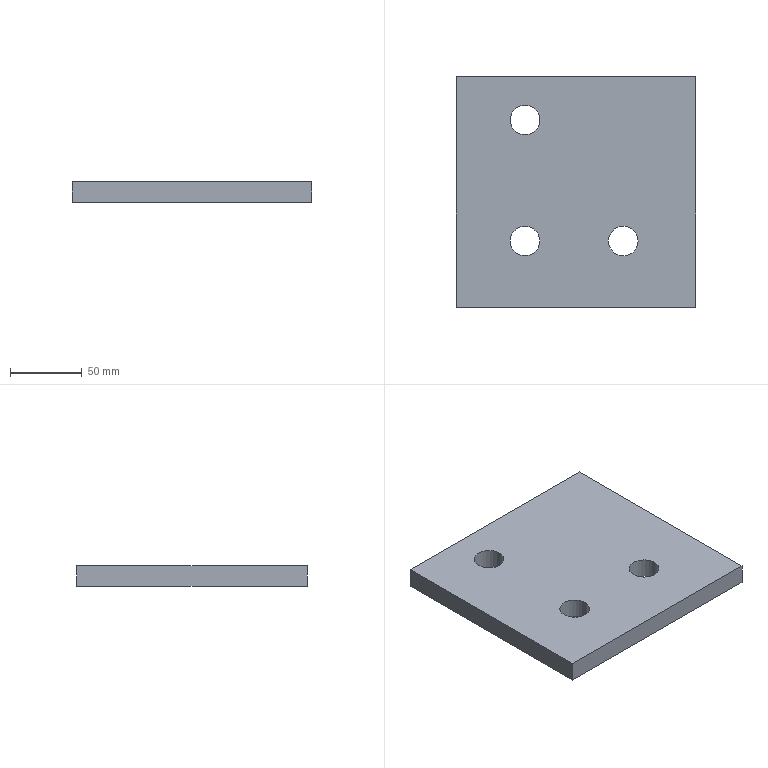Part | SolidWorks | features Extrusion 1 | 1 solid | 12 faces | box 166.35 x 160 x 14 mm | volume 358558 mm3 | cylinder 6 | plane 6 | commonest cylinder face diameters 20.65 x6
STEP:
#1=CARTESIAN_POINT('',(22.527,-34.102,14.));
#2=VERTEX_POINT('',#1);
#3=CARTESIAN_POINT('',(43.177,-34.102,14.));
#4=VERTEX_POINT('',#3);
#5=CARTESIAN_POINT('',(32.852,-34.102,14.));
#6=DIRECTION('',(0.,0.,1.));
#7=DIRECTION('',(1.,0.,0.));
#8=AXIS2_PLACEMENT_3D('',#5,#6,#7);
#9=CIRCLE('',#8,10.325);
#10=EDGE_CURVE('',#2,#4,#9,.T.);
#11=ORIENTED_EDGE('',*,*,#10,.T.);
#12=CARTESIAN_POINT('',(43.177,-34.102,0.));
#13=VERTEX_POINT('',#12);
#14=CARTESIAN_POINT('',(43.177,-34.102,14.));
#15=DIRECTION('',(0.,0.,-1.));
#16=VECTOR('',#15,1000.);
#17=LINE('',#14,#16);
#18=EDGE_CURVE('',#4,#13,#17,.T.);
#19=ORIENTED_EDGE('',*,*,#18,.T.);
#20=CARTESIAN_POINT('',(22.527,-34.102,0.));
#21=VERTEX_POINT('',#20);
#22=CARTESIAN_POINT('',(32.852,-34.102,0.));
#23=DIRECTION('',(0.,0.,1.));
#24=DIRECTION('',(1.,0.,0.));
#25=AXIS2_PLACEMENT_3D('',#22,#23,#24);
#26=CIRCLE('',#25,10.325);
#27=EDGE_CURVE('',#21,#13,#26,.T.);
#28=ORIENTED_EDGE('',*,*,#27,.F.);
#29=CARTESIAN_POINT('',(22.527,-34.102,14.));
#30=DIRECTION('',(0.,0.,-1.));
#31=VECTOR('',#30,1000.);
#32=LINE('',#29,#31);
#33=EDGE_CURVE('',#2,#21,#32,.T.);
#34=ORIENTED_EDGE('',*,*,#33,.F.);
#35=EDGE_LOOP('',(#11,#19,#28,#34));
#36=FACE_OUTER_BOUND('',#35,.T.);
#37=CARTESIAN_POINT('',(32.852,-34.102,14.));
#38=DIRECTION('',(0.,0.,-1.));
#39=DIRECTION('',(-1.,0.,0.));
#40=AXIS2_PLACEMENT_3D('',#37,#38,#39);
#41=CYLINDRICAL_SURFACE('',#40,10.325);
#42=ADVANCED_FACE('',(#36),#41,.F.);
#43=CARTESIAN_POINT('',(-45.78,-34.102,14.));
#44=VERTEX_POINT('',#43);
#45=CARTESIAN_POINT('',(-25.13,-34.102,14.));
#46=VERTEX_POINT('',#45);
#47=CARTESIAN_POINT('',(-35.455,-34.102,14.));
#48=DIRECTION('',(0.,0.,1.));
#49=DIRECTION('',(1.,0.,0.));
#50=AXIS2_PLACEMENT_3D('',#47,#48,#49);
#51=CIRCLE('',#50,10.325);
#52=EDGE_CURVE('',#44,#46,#51,.T.);
#53=ORIENTED_EDGE('',*,*,#52,.T.);
#54=CARTESIAN_POINT('',(-25.13,-34.102,0.));
#55=VERTEX_POINT('',#54);
#56=CARTESIAN_POINT('',(-25.13,-34.102,14.));
#57=DIRECTION('',(0.,0.,-1.));
#58=VECTOR('',#57,1000.);
#59=LINE('',#56,#58);
#60=EDGE_CURVE('',#46,#55,#59,.T.);
#61=ORIENTED_EDGE('',*,*,#60,.T.);
#62=CARTESIAN_POINT('',(-45.78,-34.102,0.));
#63=VERTEX_POINT('',#62);
#64=CARTESIAN_POINT('',(-35.455,-34.102,0.));
#65=DIRECTION('',(0.,0.,1.));
#66=DIRECTION('',(1.,0.,0.));
#67=AXIS2_PLACEMENT_3D('',#64,#65,#66);
#68=CIRCLE('',#67,10.325);
#69=EDGE_CURVE('',#63,#55,#68,.T.);
#70=ORIENTED_EDGE('',*,*,#69,.F.);
#71=CARTESIAN_POINT('',(-45.78,-34.102,14.));
#72=DIRECTION('',(0.,0.,-1.));
#73=VECTOR('',#72,1000.);
#74=LINE('',#71,#73);
#75=EDGE_CURVE('',#44,#63,#74,.T.);
#76=ORIENTED_EDGE('',*,*,#75,.F.);
#77=EDGE_LOOP('',(#53,#61,#70,#76));
#78=FACE_OUTER_BOUND('',#77,.T.);
#79=CARTESIAN_POINT('',(-35.455,-34.102,14.));
#80=DIRECTION('',(0.,0.,-1.));
#81=DIRECTION('',(-1.,0.,0.));
#82=AXIS2_PLACEMENT_3D('',#79,#80,#81);
#83=CYLINDRICAL_SURFACE('',#82,10.325);
#84=ADVANCED_FACE('',(#78),#83,.F.);
#85=CARTESIAN_POINT('',(-45.748,50.048,14.));
#86=VERTEX_POINT('',#85);
#87=CARTESIAN_POINT('',(-25.098,50.048,14.));
#88=VERTEX_POINT('',#87);
#89=CARTESIAN_POINT('',(-35.423,50.048,14.));
#90=DIRECTION('',(0.,0.,1.));
#91=DIRECTION('',(1.,0.,0.));
#92=AXIS2_PLACEMENT_3D('',#89,#90,#91);
#93=CIRCLE('',#92,10.325);
#94=EDGE_CURVE('',#86,#88,#93,.T.);
#95=ORIENTED_EDGE('',*,*,#94,.T.);
#96=CARTESIAN_POINT('',(-25.098,50.048,0.));
#97=VERTEX_POINT('',#96);
#98=CARTESIAN_POINT('',(-25.098,50.048,14.));
#99=DIRECTION('',(0.,0.,-1.));
#100=VECTOR('',#99,1000.);
#101=LINE('',#98,#100);
#102=EDGE_CURVE('',#88,#97,#101,.T.);
#103=ORIENTED_EDGE('',*,*,#102,.T.);
#104=CARTESIAN_POINT('',(-45.748,50.048,0.));
#105=VERTEX_POINT('',#104);
#106=CARTESIAN_POINT('',(-35.423,50.048,0.));
#107=DIRECTION('',(0.,0.,1.));
#108=DIRECTION('',(1.,0.,0.));
#109=AXIS2_PLACEMENT_3D('',#106,#107,#108);
#110=CIRCLE('',#109,10.325);
#111=EDGE_CURVE('',#105,#97,#110,.T.);
#112=ORIENTED_EDGE('',*,*,#111,.F.);
#113=CARTESIAN_POINT('',(-45.748,50.048,14.));
#114=DIRECTION('',(0.,0.,-1.));
#115=VECTOR('',#114,1000.);
#116=LINE('',#113,#115);
#117=EDGE_CURVE('',#86,#105,#116,.T.);
#118=ORIENTED_EDGE('',*,*,#117,.F.);
#119=EDGE_LOOP('',(#95,#103,#112,#118));
#120=FACE_OUTER_BOUND('',#119,.T.);
#121=CARTESIAN_POINT('',(-35.423,50.048,14.));
#122=DIRECTION('',(0.,0.,-1.));
#123=DIRECTION('',(-1.,0.,0.));
#124=AXIS2_PLACEMENT_3D('',#121,#122,#123);
#125=CYLINDRICAL_SURFACE('',#124,10.325);
#126=ADVANCED_FACE('',(#120),#125,.F.);
#127=ORIENTED_EDGE('',*,*,#52,.F.);
#128=CARTESIAN_POINT('',(-35.455,-34.102,14.));
#129=DIRECTION('',(0.,0.,1.));
#130=DIRECTION('',(1.,0.,0.));
#131=AXIS2_PLACEMENT_3D('',#128,#129,#130);
#132=CIRCLE('',#131,10.325);
#133=EDGE_CURVE('',#46,#44,#132,.T.);
#134=ORIENTED_EDGE('',*,*,#133,.F.);
#135=EDGE_LOOP('',(#127,#134));
#136=FACE_BOUND('',#135,.T.);
#137=CARTESIAN_POINT('',(83.175,-80.,14.));
#138=VERTEX_POINT('',#137);
#139=CARTESIAN_POINT('',(83.175,80.,14.));
#140=VERTEX_POINT('',#139);
#141=CARTESIAN_POINT('',(83.175,80.,14.));
#142=DIRECTION('',(0.,1.,0.));
#143=VECTOR('',#142,1000.);
#144=LINE('',#141,#143);
#145=EDGE_CURVE('',#138,#140,#144,.T.);
#146=ORIENTED_EDGE('',*,*,#145,.T.);
#147=CARTESIAN_POINT('',(-83.175,80.,14.));
#148=VERTEX_POINT('',#147);
#149=CARTESIAN_POINT('',(-83.175,80.,14.));
#150=DIRECTION('',(-1.,0.,0.));
#151=VECTOR('',#150,1000.);
#152=LINE('',#149,#151);
#153=EDGE_CURVE('',#140,#148,#152,.T.);
#154=ORIENTED_EDGE('',*,*,#153,.T.);
#155=CARTESIAN_POINT('',(-83.175,-80.,14.));
#156=VERTEX_POINT('',#155);
#157=CARTESIAN_POINT('',(-83.175,80.,14.));
#158=DIRECTION('',(0.,-1.,0.));
#159=VECTOR('',#158,1000.);
#160=LINE('',#157,#159);
#161=EDGE_CURVE('',#148,#156,#160,.T.);
#162=ORIENTED_EDGE('',*,*,#161,.T.);
#163=CARTESIAN_POINT('',(-83.175,-80.,14.));
#164=DIRECTION('',(1.,0.,0.));
#165=VECTOR('',#164,1000.);
#166=LINE('',#163,#165);
#167=EDGE_CURVE('',#156,#138,#166,.T.);
#168=ORIENTED_EDGE('',*,*,#167,.T.);
#169=EDGE_LOOP('',(#146,#154,#162,#168));
#170=FACE_OUTER_BOUND('',#169,.T.);
#171=ORIENTED_EDGE('',*,*,#94,.F.);
#172=CARTESIAN_POINT('',(-35.423,50.048,14.));
#173=DIRECTION('',(0.,0.,1.));
#174=DIRECTION('',(1.,0.,0.));
#175=AXIS2_PLACEMENT_3D('',#172,#173,#174);
#176=CIRCLE('',#175,10.325);
#177=EDGE_CURVE('',#88,#86,#176,.T.);
#178=ORIENTED_EDGE('',*,*,#177,.F.);
#179=EDGE_LOOP('',(#171,#178));
#180=FACE_BOUND('',#179,.T.);
#181=ORIENTED_EDGE('',*,*,#10,.F.);
#182=CARTESIAN_POINT('',(32.852,-34.102,14.));
#183=DIRECTION('',(0.,0.,1.));
#184=DIRECTION('',(1.,0.,0.));
#185=AXIS2_PLACEMENT_3D('',#182,#183,#184);
#186=CIRCLE('',#185,10.325);
#187=EDGE_CURVE('',#4,#2,#186,.T.);
#188=ORIENTED_EDGE('',*,*,#187,.F.);
#189=EDGE_LOOP('',(#181,#188));
#190=FACE_BOUND('',#189,.T.);
#191=CARTESIAN_POINT('',(83.175,-80.,14.));
#192=DIRECTION('',(0.,0.,1.));
#193=DIRECTION('',(1.,0.,0.));
#194=AXIS2_PLACEMENT_3D('',#191,#192,#193);
#195=PLANE('',#194);
#196=ADVANCED_FACE('',(#136,#170,#180,#190),#195,.T.);
#197=ORIENTED_EDGE('',*,*,#69,.T.);
#198=CARTESIAN_POINT('',(-35.455,-34.102,0.));
#199=DIRECTION('',(0.,0.,1.));
#200=DIRECTION('',(1.,0.,0.));
#201=AXIS2_PLACEMENT_3D('',#198,#199,#200);
#202=CIRCLE('',#201,10.325);
#203=EDGE_CURVE('',#55,#63,#202,.T.);
#204=ORIENTED_EDGE('',*,*,#203,.T.);
#205=EDGE_LOOP('',(#197,#204));
#206=FACE_BOUND('',#205,.T.);
#207=CARTESIAN_POINT('',(83.175,-80.,0.));
#208=VERTEX_POINT('',#207);
#209=CARTESIAN_POINT('',(83.175,80.,0.));
#210=VERTEX_POINT('',#209);
#211=CARTESIAN_POINT('',(83.175,80.,0.));
#212=DIRECTION('',(0.,1.,0.));
#213=VECTOR('',#212,1000.);
#214=LINE('',#211,#213);
#215=EDGE_CURVE('',#208,#210,#214,.T.);
#216=ORIENTED_EDGE('',*,*,#215,.F.);
#217=CARTESIAN_POINT('',(-83.175,-80.,0.));
#218=VERTEX_POINT('',#217);
#219=CARTESIAN_POINT('',(-83.175,-80.,0.));
#220=DIRECTION('',(1.,0.,0.));
#221=VECTOR('',#220,1000.);
#222=LINE('',#219,#221);
#223=EDGE_CURVE('',#218,#208,#222,.T.);
#224=ORIENTED_EDGE('',*,*,#223,.F.);
#225=CARTESIAN_POINT('',(-83.175,80.,0.));
#226=VERTEX_POINT('',#225);
#227=CARTESIAN_POINT('',(-83.175,80.,0.));
#228=DIRECTION('',(0.,-1.,0.));
#229=VECTOR('',#228,1000.);
#230=LINE('',#227,#229);
#231=EDGE_CURVE('',#226,#218,#230,.T.);
#232=ORIENTED_EDGE('',*,*,#231,.F.);
#233=CARTESIAN_POINT('',(-83.175,80.,0.));
#234=DIRECTION('',(-1.,0.,0.));
#235=VECTOR('',#234,1000.);
#236=LINE('',#233,#235);
#237=EDGE_CURVE('',#210,#226,#236,.T.);
#238=ORIENTED_EDGE('',*,*,#237,.F.);
#239=EDGE_LOOP('',(#216,#224,#232,#238));
#240=FACE_OUTER_BOUND('',#239,.T.);
#241=ORIENTED_EDGE('',*,*,#111,.T.);
#242=CARTESIAN_POINT('',(-35.423,50.048,0.));
#243=DIRECTION('',(0.,0.,1.));
#244=DIRECTION('',(1.,0.,0.));
#245=AXIS2_PLACEMENT_3D('',#242,#243,#244);
#246=CIRCLE('',#245,10.325);
#247=EDGE_CURVE('',#97,#105,#246,.T.);
#248=ORIENTED_EDGE('',*,*,#247,.T.);
#249=EDGE_LOOP('',(#241,#248));
#250=FACE_BOUND('',#249,.T.);
#251=ORIENTED_EDGE('',*,*,#27,.T.);
#252=CARTESIAN_POINT('',(32.852,-34.102,0.));
#253=DIRECTION('',(0.,0.,1.));
#254=DIRECTION('',(1.,0.,0.));
#255=AXIS2_PLACEMENT_3D('',#252,#253,#254);
#256=CIRCLE('',#255,10.325);
#257=EDGE_CURVE('',#13,#21,#256,.T.);
#258=ORIENTED_EDGE('',*,*,#257,.T.);
#259=EDGE_LOOP('',(#251,#258));
#260=FACE_BOUND('',#259,.T.);
#261=CARTESIAN_POINT('',(83.175,-80.,0.));
#262=DIRECTION('',(0.,0.,1.));
#263=DIRECTION('',(1.,0.,0.));
#264=AXIS2_PLACEMENT_3D('',#261,#262,#263);
#265=PLANE('',#264);
#266=ADVANCED_FACE('',(#206,#240,#250,#260),#265,.F.);
#267=ORIENTED_EDGE('',*,*,#215,.T.);
#268=CARTESIAN_POINT('',(83.175,80.,14.));
#269=DIRECTION('',(0.,0.,-1.));
#270=VECTOR('',#269,1000.);
#271=LINE('',#268,#270);
#272=EDGE_CURVE('',#140,#210,#271,.T.);
#273=ORIENTED_EDGE('',*,*,#272,.F.);
#274=ORIENTED_EDGE('',*,*,#145,.F.);
#275=CARTESIAN_POINT('',(83.175,-80.,14.));
#276=DIRECTION('',(0.,0.,-1.));
#277=VECTOR('',#276,1000.);
#278=LINE('',#275,#277);
#279=EDGE_CURVE('',#138,#208,#278,.T.);
#280=ORIENTED_EDGE('',*,*,#279,.T.);
#281=EDGE_LOOP('',(#267,#273,#274,#280));
#282=FACE_OUTER_BOUND('',#281,.T.);
#283=CARTESIAN_POINT('',(83.175,80.,14.));
#284=DIRECTION('',(-1.,0.,0.));
#285=DIRECTION('',(0.,-1.,0.));
#286=AXIS2_PLACEMENT_3D('',#283,#284,#285);
#287=PLANE('',#286);
#288=ADVANCED_FACE('',(#282),#287,.F.);
#289=ORIENTED_EDGE('',*,*,#237,.T.);
#290=CARTESIAN_POINT('',(-83.175,80.,14.));
#291=DIRECTION('',(0.,0.,-1.));
#292=VECTOR('',#291,1000.);
#293=LINE('',#290,#292);
#294=EDGE_CURVE('',#148,#226,#293,.T.);
#295=ORIENTED_EDGE('',*,*,#294,.F.);
#296=ORIENTED_EDGE('',*,*,#153,.F.);
#297=ORIENTED_EDGE('',*,*,#272,.T.);
#298=EDGE_LOOP('',(#289,#295,#296,#297));
#299=FACE_OUTER_BOUND('',#298,.T.);
#300=CARTESIAN_POINT('',(-83.175,80.,14.));
#301=DIRECTION('',(0.,-1.,0.));
#302=DIRECTION('',(0.,0.,-1.));
#303=AXIS2_PLACEMENT_3D('',#300,#301,#302);
#304=PLANE('',#303);
#305=ADVANCED_FACE('',(#299),#304,.F.);
#306=ORIENTED_EDGE('',*,*,#231,.T.);
#307=CARTESIAN_POINT('',(-83.175,-80.,14.));
#308=DIRECTION('',(0.,0.,-1.));
#309=VECTOR('',#308,1000.);
#310=LINE('',#307,#309);
#311=EDGE_CURVE('',#156,#218,#310,.T.);
#312=ORIENTED_EDGE('',*,*,#311,.F.);
#313=ORIENTED_EDGE('',*,*,#161,.F.);
#314=ORIENTED_EDGE('',*,*,#294,.T.);
#315=EDGE_LOOP('',(#306,#312,#313,#314));
#316=FACE_OUTER_BOUND('',#315,.T.);
#317=CARTESIAN_POINT('',(-83.175,80.,14.));
#318=DIRECTION('',(1.,0.,0.));
#319=DIRECTION('',(0.,1.,0.));
#320=AXIS2_PLACEMENT_3D('',#317,#318,#319);
#321=PLANE('',#320);
#322=ADVANCED_FACE('',(#316),#321,.F.);
#323=ORIENTED_EDGE('',*,*,#223,.T.);
#324=ORIENTED_EDGE('',*,*,#279,.F.);
#325=ORIENTED_EDGE('',*,*,#167,.F.);
#326=ORIENTED_EDGE('',*,*,#311,.T.);
#327=EDGE_LOOP('',(#323,#324,#325,#326));
#328=FACE_OUTER_BOUND('',#327,.T.);
#329=CARTESIAN_POINT('',(-83.175,-80.,14.));
#330=DIRECTION('',(0.,1.,0.));
#331=DIRECTION('',(0.,0.,1.));
#332=AXIS2_PLACEMENT_3D('',#329,#330,#331);
#333=PLANE('',#332);
#334=ADVANCED_FACE('',(#328),#333,.F.);
#335=ORIENTED_EDGE('',*,*,#102,.F.);
#336=ORIENTED_EDGE('',*,*,#177,.T.);
#337=ORIENTED_EDGE('',*,*,#117,.T.);
#338=ORIENTED_EDGE('',*,*,#247,.F.);
#339=EDGE_LOOP('',(#335,#336,#337,#338));
#340=FACE_OUTER_BOUND('',#339,.T.);
#341=CARTESIAN_POINT('',(-35.423,50.048,14.));
#342=DIRECTION('',(0.,0.,-1.));
#343=DIRECTION('',(-1.,0.,0.));
#344=AXIS2_PLACEMENT_3D('',#341,#342,#343);
#345=CYLINDRICAL_SURFACE('',#344,10.325);
#346=ADVANCED_FACE('',(#340),#345,.F.);
#347=ORIENTED_EDGE('',*,*,#60,.F.);
#348=ORIENTED_EDGE('',*,*,#133,.T.);
#349=ORIENTED_EDGE('',*,*,#75,.T.);
#350=ORIENTED_EDGE('',*,*,#203,.F.);
#351=EDGE_LOOP('',(#347,#348,#349,#350));
#352=FACE_OUTER_BOUND('',#351,.T.);
#353=CARTESIAN_POINT('',(-35.455,-34.102,14.));
#354=DIRECTION('',(0.,0.,-1.));
#355=DIRECTION('',(-1.,0.,0.));
#356=AXIS2_PLACEMENT_3D('',#353,#354,#355);
#357=CYLINDRICAL_SURFACE('',#356,10.325);
#358=ADVANCED_FACE('',(#352),#357,.F.);
#359=ORIENTED_EDGE('',*,*,#18,.F.);
#360=ORIENTED_EDGE('',*,*,#187,.T.);
#361=ORIENTED_EDGE('',*,*,#33,.T.);
#362=ORIENTED_EDGE('',*,*,#257,.F.);
#363=EDGE_LOOP('',(#359,#360,#361,#362));
#364=FACE_OUTER_BOUND('',#363,.T.);
#365=CARTESIAN_POINT('',(32.852,-34.102,14.));
#366=DIRECTION('',(0.,0.,-1.));
#367=DIRECTION('',(-1.,0.,0.));
#368=AXIS2_PLACEMENT_3D('',#365,#366,#367);
#369=CYLINDRICAL_SURFACE('',#368,10.325);
#370=ADVANCED_FACE('',(#364),#369,.F.);
#371=CLOSED_SHELL('',(#42,#84,#126,#196,#266,#288,#305,#322,#334,#346,#358,#370));
#372=MANIFOLD_SOLID_BREP('',#371);
#373=CARTESIAN_POINT('',(0.,0.,0.));
#374=DIRECTION('',(0.,0.,1.));
#375=DIRECTION('',(1.,0.,0.));
#376=AXIS2_PLACEMENT_3D('',#373,#374,#375);
#377=(LENGTH_UNIT()NAMED_UNIT(*)SI_UNIT(.MILLI.,.METRE.));
#378=UNCERTAINTY_MEASURE_WITH_UNIT(LENGTH_MEASURE(0.00001),#377,'','');
#379=(NAMED_UNIT(*)PLANE_ANGLE_UNIT()SI_UNIT($,.RADIAN.));
#380=(NAMED_UNIT(*)SI_UNIT($,.STERADIAN.)SOLID_ANGLE_UNIT());
#381=(GEOMETRIC_REPRESENTATION_CONTEXT(3)GLOBAL_UNCERTAINTY_ASSIGNED_CONTEXT((#378))GLOBAL_UNIT_ASSIGNED_CONTEXT((#377,#379,#380))REPRESENTATION_CONTEXT('',''));
#382=ADVANCED_BREP_SHAPE_REPRESENTATION('',(#372,#376),#381);